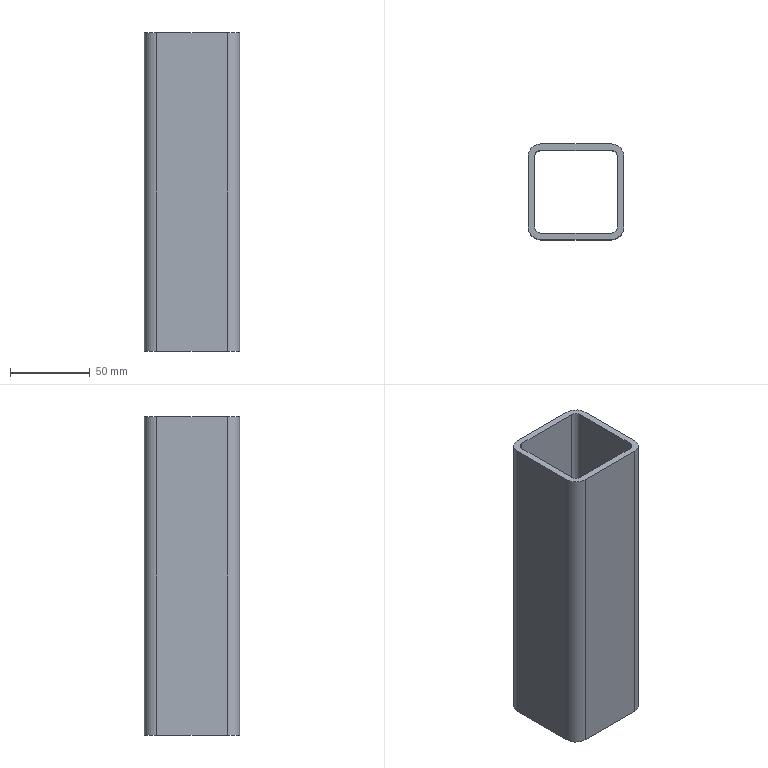Part | SolidWorks | features BaseBody 1 | 1 solid | 18 faces | box 60 x 60 x 200 mm | volume 170959 mm3 | plane 10 | cylinder 8 | commonest cylinder face diameters 8 x4 16 x4
STEP:
#1=CARTESIAN_POINT('',(696.,2440.,-1360.));
#2=VERTEX_POINT('',#1);
#3=CARTESIAN_POINT('',(696.,2484.,-1360.));
#4=VERTEX_POINT('',#3);
#5=CARTESIAN_POINT('',(696.,2440.,-1360.));
#6=DIRECTION('',(0.,1.,0.));
#7=VECTOR('',#6,1000.);
#8=LINE('',#5,#7);
#9=EDGE_CURVE('',#2,#4,#8,.T.);
#10=ORIENTED_EDGE('',*,*,#9,.T.);
#11=CARTESIAN_POINT('',(696.,2484.,-1560.));
#12=VERTEX_POINT('',#11);
#13=CARTESIAN_POINT('',(696.,2484.,-1530.));
#14=DIRECTION('',(0.,0.,-1.));
#15=VECTOR('',#14,1000.);
#16=LINE('',#13,#15);
#17=EDGE_CURVE('',#4,#12,#16,.T.);
#18=ORIENTED_EDGE('',*,*,#17,.T.);
#19=CARTESIAN_POINT('',(696.,2440.,-1560.));
#20=VERTEX_POINT('',#19);
#21=CARTESIAN_POINT('',(696.,2440.,-1560.));
#22=DIRECTION('',(0.,-1.,0.));
#23=VECTOR('',#22,1000.);
#24=LINE('',#21,#23);
#25=EDGE_CURVE('',#12,#20,#24,.T.);
#26=ORIENTED_EDGE('',*,*,#25,.T.);
#27=CARTESIAN_POINT('',(696.,2440.,-1530.));
#28=DIRECTION('',(0.,0.,1.));
#29=VECTOR('',#28,1000.);
#30=LINE('',#27,#29);
#31=EDGE_CURVE('',#20,#2,#30,.T.);
#32=ORIENTED_EDGE('',*,*,#31,.T.);
#33=EDGE_LOOP('',(#10,#18,#26,#32));
#34=FACE_OUTER_BOUND('',#33,.T.);
#35=CARTESIAN_POINT('',(696.,2440.,-1530.));
#36=DIRECTION('',(-1.,0.,0.));
#37=DIRECTION('',(0.,0.,1.));
#38=AXIS2_PLACEMENT_3D('',#35,#36,#37);
#39=PLANE('',#38);
#40=ADVANCED_FACE('',(#34),#39,.T.);
#41=ORIENTED_EDGE('',*,*,#17,.F.);
#42=CARTESIAN_POINT('',(692.,2488.,-1360.));
#43=VERTEX_POINT('',#42);
#44=CARTESIAN_POINT('',(692.,2484.,-1360.));
#45=DIRECTION('',(0.,0.,-1.));
#46=DIRECTION('',(1.,0.,0.));
#47=AXIS2_PLACEMENT_3D('',#44,#45,#46);
#48=CIRCLE('',#47,4.);
#49=EDGE_CURVE('',#43,#4,#48,.T.);
#50=ORIENTED_EDGE('',*,*,#49,.F.);
#51=CARTESIAN_POINT('',(692.,2488.,-1560.));
#52=VERTEX_POINT('',#51);
#53=CARTESIAN_POINT('',(692.,2488.,-1530.));
#54=DIRECTION('',(0.,0.,1.));
#55=VECTOR('',#54,1000.);
#56=LINE('',#53,#55);
#57=EDGE_CURVE('',#52,#43,#56,.T.);
#58=ORIENTED_EDGE('',*,*,#57,.F.);
#59=CARTESIAN_POINT('',(692.,2484.,-1560.));
#60=DIRECTION('',(0.,0.,1.));
#61=DIRECTION('',(1.,0.,0.));
#62=AXIS2_PLACEMENT_3D('',#59,#60,#61);
#63=CIRCLE('',#62,4.);
#64=EDGE_CURVE('',#12,#52,#63,.T.);
#65=ORIENTED_EDGE('',*,*,#64,.F.);
#66=EDGE_LOOP('',(#41,#50,#58,#65));
#67=FACE_OUTER_BOUND('',#66,.T.);
#68=CARTESIAN_POINT('',(692.,2484.,-1530.));
#69=DIRECTION('',(0.,0.,1.));
#70=DIRECTION('',(1.,0.,0.));
#71=AXIS2_PLACEMENT_3D('',#68,#69,#70);
#72=CYLINDRICAL_SURFACE('',#71,4.);
#73=ADVANCED_FACE('',(#67),#72,.F.);
#74=CARTESIAN_POINT('',(692.,2436.,-1360.));
#75=VERTEX_POINT('',#74);
#76=CARTESIAN_POINT('',(692.,2440.,-1360.));
#77=DIRECTION('',(0.,0.,1.));
#78=DIRECTION('',(1.,0.,0.));
#79=AXIS2_PLACEMENT_3D('',#76,#77,#78);
#80=CIRCLE('',#79,4.);
#81=EDGE_CURVE('',#75,#2,#80,.T.);
#82=ORIENTED_EDGE('',*,*,#81,.F.);
#83=CARTESIAN_POINT('',(648.,2436.,-1360.));
#84=VERTEX_POINT('',#83);
#85=CARTESIAN_POINT('',(-670.,2436.,-1360.));
#86=DIRECTION('',(1.,0.,0.));
#87=VECTOR('',#86,1000.);
#88=LINE('',#85,#87);
#89=EDGE_CURVE('',#84,#75,#88,.T.);
#90=ORIENTED_EDGE('',*,*,#89,.F.);
#91=CARTESIAN_POINT('',(644.,2440.,-1360.));
#92=VERTEX_POINT('',#91);
#93=CARTESIAN_POINT('',(648.,2440.,-1360.));
#94=DIRECTION('',(0.,0.,1.));
#95=DIRECTION('',(1.,0.,0.));
#96=AXIS2_PLACEMENT_3D('',#93,#94,#95);
#97=CIRCLE('',#96,4.);
#98=EDGE_CURVE('',#92,#84,#97,.T.);
#99=ORIENTED_EDGE('',*,*,#98,.F.);
#100=CARTESIAN_POINT('',(644.,2484.,-1360.));
#101=VERTEX_POINT('',#100);
#102=CARTESIAN_POINT('',(644.,1242.,-1360.));
#103=DIRECTION('',(0.,-1.,0.));
#104=VECTOR('',#103,1000.);
#105=LINE('',#102,#104);
#106=EDGE_CURVE('',#101,#92,#105,.T.);
#107=ORIENTED_EDGE('',*,*,#106,.F.);
#108=CARTESIAN_POINT('',(648.,2488.,-1360.));
#109=VERTEX_POINT('',#108);
#110=CARTESIAN_POINT('',(648.,2484.,-1360.));
#111=DIRECTION('',(0.,0.,1.));
#112=DIRECTION('',(1.,0.,0.));
#113=AXIS2_PLACEMENT_3D('',#110,#111,#112);
#114=CIRCLE('',#113,4.);
#115=EDGE_CURVE('',#109,#101,#114,.T.);
#116=ORIENTED_EDGE('',*,*,#115,.F.);
#117=CARTESIAN_POINT('',(-670.,2488.,-1360.));
#118=DIRECTION('',(-1.,0.,0.));
#119=VECTOR('',#118,1000.);
#120=LINE('',#117,#119);
#121=EDGE_CURVE('',#43,#109,#120,.T.);
#122=ORIENTED_EDGE('',*,*,#121,.F.);
#123=ORIENTED_EDGE('',*,*,#49,.T.);
#124=ORIENTED_EDGE('',*,*,#9,.F.);
#125=EDGE_LOOP('',(#82,#90,#99,#107,#116,#122,#123,#124));
#126=FACE_BOUND('',#125,.T.);
#127=CARTESIAN_POINT('',(692.,2432.,-1360.));
#128=VERTEX_POINT('',#127);
#129=CARTESIAN_POINT('',(648.,2432.,-1360.));
#130=VERTEX_POINT('',#129);
#131=CARTESIAN_POINT('',(-670.,2432.,-1360.));
#132=DIRECTION('',(-1.,0.,0.));
#133=VECTOR('',#132,1000.);
#134=LINE('',#131,#133);
#135=EDGE_CURVE('',#128,#130,#134,.T.);
#136=ORIENTED_EDGE('',*,*,#135,.F.);
#137=CARTESIAN_POINT('',(700.,2440.,-1360.));
#138=VERTEX_POINT('',#137);
#139=CARTESIAN_POINT('',(692.,2440.,-1360.));
#140=DIRECTION('',(0.,0.,-1.));
#141=DIRECTION('',(1.,0.,0.));
#142=AXIS2_PLACEMENT_3D('',#139,#140,#141);
#143=CIRCLE('',#142,8.);
#144=EDGE_CURVE('',#138,#128,#143,.T.);
#145=ORIENTED_EDGE('',*,*,#144,.F.);
#146=CARTESIAN_POINT('',(700.,2484.,-1360.));
#147=VERTEX_POINT('',#146);
#148=CARTESIAN_POINT('',(700.,1242.,-1360.));
#149=DIRECTION('',(0.,-1.,0.));
#150=VECTOR('',#149,1000.);
#151=LINE('',#148,#150);
#152=EDGE_CURVE('',#147,#138,#151,.T.);
#153=ORIENTED_EDGE('',*,*,#152,.F.);
#154=CARTESIAN_POINT('',(692.,2492.,-1360.));
#155=VERTEX_POINT('',#154);
#156=CARTESIAN_POINT('',(692.,2484.,-1360.));
#157=DIRECTION('',(0.,0.,-1.));
#158=DIRECTION('',(1.,0.,0.));
#159=AXIS2_PLACEMENT_3D('',#156,#157,#158);
#160=CIRCLE('',#159,8.);
#161=EDGE_CURVE('',#155,#147,#160,.T.);
#162=ORIENTED_EDGE('',*,*,#161,.F.);
#163=CARTESIAN_POINT('',(648.,2492.,-1360.));
#164=VERTEX_POINT('',#163);
#165=CARTESIAN_POINT('',(-670.,2492.,-1360.));
#166=DIRECTION('',(1.,0.,0.));
#167=VECTOR('',#166,1000.);
#168=LINE('',#165,#167);
#169=EDGE_CURVE('',#164,#155,#168,.T.);
#170=ORIENTED_EDGE('',*,*,#169,.F.);
#171=CARTESIAN_POINT('',(640.,2484.,-1360.));
#172=VERTEX_POINT('',#171);
#173=CARTESIAN_POINT('',(648.,2484.,-1360.));
#174=DIRECTION('',(0.,0.,-1.));
#175=DIRECTION('',(1.,0.,0.));
#176=AXIS2_PLACEMENT_3D('',#173,#174,#175);
#177=CIRCLE('',#176,8.);
#178=EDGE_CURVE('',#172,#164,#177,.T.);
#179=ORIENTED_EDGE('',*,*,#178,.F.);
#180=CARTESIAN_POINT('',(640.,2440.,-1360.));
#181=VERTEX_POINT('',#180);
#182=CARTESIAN_POINT('',(640.,1242.,-1360.));
#183=DIRECTION('',(0.,1.,0.));
#184=VECTOR('',#183,1000.);
#185=LINE('',#182,#184);
#186=EDGE_CURVE('',#181,#172,#185,.T.);
#187=ORIENTED_EDGE('',*,*,#186,.F.);
#188=CARTESIAN_POINT('',(648.,2440.,-1360.));
#189=DIRECTION('',(0.,0.,-1.));
#190=DIRECTION('',(1.,0.,0.));
#191=AXIS2_PLACEMENT_3D('',#188,#189,#190);
#192=CIRCLE('',#191,8.);
#193=EDGE_CURVE('',#130,#181,#192,.T.);
#194=ORIENTED_EDGE('',*,*,#193,.F.);
#195=EDGE_LOOP('',(#136,#145,#153,#162,#170,#179,#187,#194));
#196=FACE_OUTER_BOUND('',#195,.T.);
#197=CARTESIAN_POINT('',(-670.,1242.,-1360.));
#198=DIRECTION('',(0.,0.,-1.));
#199=DIRECTION('',(-1.,0.,0.));
#200=AXIS2_PLACEMENT_3D('',#197,#198,#199);
#201=PLANE('',#200);
#202=ADVANCED_FACE('',(#126,#196),#201,.F.);
#203=CARTESIAN_POINT('',(692.,2436.,-1560.));
#204=VERTEX_POINT('',#203);
#205=CARTESIAN_POINT('',(692.,2436.,-1530.));
#206=DIRECTION('',(0.,0.,-1.));
#207=VECTOR('',#206,1000.);
#208=LINE('',#205,#207);
#209=EDGE_CURVE('',#75,#204,#208,.T.);
#210=ORIENTED_EDGE('',*,*,#209,.F.);
#211=ORIENTED_EDGE('',*,*,#81,.T.);
#212=ORIENTED_EDGE('',*,*,#31,.F.);
#213=CARTESIAN_POINT('',(692.,2440.,-1560.));
#214=DIRECTION('',(0.,0.,1.));
#215=DIRECTION('',(1.,0.,0.));
#216=AXIS2_PLACEMENT_3D('',#213,#214,#215);
#217=CIRCLE('',#216,4.);
#218=EDGE_CURVE('',#204,#20,#217,.T.);
#219=ORIENTED_EDGE('',*,*,#218,.F.);
#220=EDGE_LOOP('',(#210,#211,#212,#219));
#221=FACE_OUTER_BOUND('',#220,.T.);
#222=CARTESIAN_POINT('',(692.,2440.,-1530.));
#223=DIRECTION('',(0.,0.,1.));
#224=DIRECTION('',(1.,0.,0.));
#225=AXIS2_PLACEMENT_3D('',#222,#223,#224);
#226=CYLINDRICAL_SURFACE('',#225,4.);
#227=ADVANCED_FACE('',(#221),#226,.F.);
#228=ORIENTED_EDGE('',*,*,#25,.F.);
#229=ORIENTED_EDGE('',*,*,#64,.T.);
#230=CARTESIAN_POINT('',(648.,2488.,-1560.));
#231=VERTEX_POINT('',#230);
#232=CARTESIAN_POINT('',(670.,2488.,-1560.));
#233=DIRECTION('',(-1.,0.,0.));
#234=VECTOR('',#233,1000.);
#235=LINE('',#232,#234);
#236=EDGE_CURVE('',#52,#231,#235,.T.);
#237=ORIENTED_EDGE('',*,*,#236,.T.);
#238=CARTESIAN_POINT('',(644.,2484.,-1560.));
#239=VERTEX_POINT('',#238);
#240=CARTESIAN_POINT('',(648.,2484.,-1560.));
#241=DIRECTION('',(0.,0.,1.));
#242=DIRECTION('',(1.,0.,0.));
#243=AXIS2_PLACEMENT_3D('',#240,#241,#242);
#244=CIRCLE('',#243,4.);
#245=EDGE_CURVE('',#231,#239,#244,.T.);
#246=ORIENTED_EDGE('',*,*,#245,.T.);
#247=CARTESIAN_POINT('',(644.,2440.,-1560.));
#248=VERTEX_POINT('',#247);
#249=CARTESIAN_POINT('',(644.,2492.,-1560.));
#250=DIRECTION('',(0.,-1.,0.));
#251=VECTOR('',#250,1000.);
#252=LINE('',#249,#251);
#253=EDGE_CURVE('',#239,#248,#252,.T.);
#254=ORIENTED_EDGE('',*,*,#253,.T.);
#255=CARTESIAN_POINT('',(648.,2436.,-1560.));
#256=VERTEX_POINT('',#255);
#257=CARTESIAN_POINT('',(648.,2440.,-1560.));
#258=DIRECTION('',(0.,0.,1.));
#259=DIRECTION('',(1.,0.,0.));
#260=AXIS2_PLACEMENT_3D('',#257,#258,#259);
#261=CIRCLE('',#260,4.);
#262=EDGE_CURVE('',#248,#256,#261,.T.);
#263=ORIENTED_EDGE('',*,*,#262,.T.);
#264=CARTESIAN_POINT('',(670.,2436.,-1560.));
#265=DIRECTION('',(1.,0.,0.));
#266=VECTOR('',#265,1000.);
#267=LINE('',#264,#266);
#268=EDGE_CURVE('',#256,#204,#267,.T.);
#269=ORIENTED_EDGE('',*,*,#268,.T.);
#270=ORIENTED_EDGE('',*,*,#218,.T.);
#271=EDGE_LOOP('',(#228,#229,#237,#246,#254,#263,#269,#270));
#272=FACE_BOUND('',#271,.T.);
#273=CARTESIAN_POINT('',(648.,2432.,-1560.));
#274=VERTEX_POINT('',#273);
#275=CARTESIAN_POINT('',(640.,2440.,-1560.));
#276=VERTEX_POINT('',#275);
#277=CARTESIAN_POINT('',(648.,2440.,-1560.));
#278=DIRECTION('',(0.,0.,-1.));
#279=DIRECTION('',(1.,0.,0.));
#280=AXIS2_PLACEMENT_3D('',#277,#278,#279);
#281=CIRCLE('',#280,8.);
#282=EDGE_CURVE('',#274,#276,#281,.T.);
#283=ORIENTED_EDGE('',*,*,#282,.T.);
#284=CARTESIAN_POINT('',(640.,2484.,-1560.));
#285=VERTEX_POINT('',#284);
#286=CARTESIAN_POINT('',(640.,2492.,-1560.));
#287=DIRECTION('',(0.,1.,0.));
#288=VECTOR('',#287,1000.);
#289=LINE('',#286,#288);
#290=EDGE_CURVE('',#276,#285,#289,.T.);
#291=ORIENTED_EDGE('',*,*,#290,.T.);
#292=CARTESIAN_POINT('',(648.,2492.,-1560.));
#293=VERTEX_POINT('',#292);
#294=CARTESIAN_POINT('',(648.,2484.,-1560.));
#295=DIRECTION('',(0.,0.,-1.));
#296=DIRECTION('',(1.,0.,0.));
#297=AXIS2_PLACEMENT_3D('',#294,#295,#296);
#298=CIRCLE('',#297,8.);
#299=EDGE_CURVE('',#285,#293,#298,.T.);
#300=ORIENTED_EDGE('',*,*,#299,.T.);
#301=CARTESIAN_POINT('',(692.,2492.,-1560.));
#302=VERTEX_POINT('',#301);
#303=CARTESIAN_POINT('',(670.,2492.,-1560.));
#304=DIRECTION('',(1.,0.,0.));
#305=VECTOR('',#304,1000.);
#306=LINE('',#303,#305);
#307=EDGE_CURVE('',#293,#302,#306,.T.);
#308=ORIENTED_EDGE('',*,*,#307,.T.);
#309=CARTESIAN_POINT('',(700.,2484.,-1560.));
#310=VERTEX_POINT('',#309);
#311=CARTESIAN_POINT('',(692.,2484.,-1560.));
#312=DIRECTION('',(0.,0.,-1.));
#313=DIRECTION('',(1.,0.,0.));
#314=AXIS2_PLACEMENT_3D('',#311,#312,#313);
#315=CIRCLE('',#314,8.);
#316=EDGE_CURVE('',#302,#310,#315,.T.);
#317=ORIENTED_EDGE('',*,*,#316,.T.);
#318=CARTESIAN_POINT('',(700.,2440.,-1560.));
#319=VERTEX_POINT('',#318);
#320=CARTESIAN_POINT('',(700.,2492.,-1560.));
#321=DIRECTION('',(0.,-1.,0.));
#322=VECTOR('',#321,1000.);
#323=LINE('',#320,#322);
#324=EDGE_CURVE('',#310,#319,#323,.T.);
#325=ORIENTED_EDGE('',*,*,#324,.T.);
#326=CARTESIAN_POINT('',(692.,2432.,-1560.));
#327=VERTEX_POINT('',#326);
#328=CARTESIAN_POINT('',(692.,2440.,-1560.));
#329=DIRECTION('',(0.,0.,-1.));
#330=DIRECTION('',(1.,0.,0.));
#331=AXIS2_PLACEMENT_3D('',#328,#329,#330);
#332=CIRCLE('',#331,8.);
#333=EDGE_CURVE('',#319,#327,#332,.T.);
#334=ORIENTED_EDGE('',*,*,#333,.T.);
#335=CARTESIAN_POINT('',(670.,2432.,-1560.));
#336=DIRECTION('',(-1.,0.,0.));
#337=VECTOR('',#336,1000.);
#338=LINE('',#335,#337);
#339=EDGE_CURVE('',#327,#274,#338,.T.);
#340=ORIENTED_EDGE('',*,*,#339,.T.);
#341=EDGE_LOOP('',(#283,#291,#300,#308,#317,#325,#334,#340));
#342=FACE_OUTER_BOUND('',#341,.T.);
#343=CARTESIAN_POINT('',(670.,2492.,-1560.));
#344=DIRECTION('',(0.,0.,-1.));
#345=DIRECTION('',(-1.,0.,0.));
#346=AXIS2_PLACEMENT_3D('',#343,#344,#345);
#347=PLANE('',#346);
#348=ADVANCED_FACE('',(#272,#342),#347,.T.);
#349=ORIENTED_EDGE('',*,*,#121,.T.);
#350=CARTESIAN_POINT('',(648.,2488.,-1530.));
#351=DIRECTION('',(0.,0.,-1.));
#352=VECTOR('',#351,1000.);
#353=LINE('',#350,#352);
#354=EDGE_CURVE('',#109,#231,#353,.T.);
#355=ORIENTED_EDGE('',*,*,#354,.T.);
#356=ORIENTED_EDGE('',*,*,#236,.F.);
#357=ORIENTED_EDGE('',*,*,#57,.T.);
#358=EDGE_LOOP('',(#349,#355,#356,#357));
#359=FACE_OUTER_BOUND('',#358,.T.);
#360=CARTESIAN_POINT('',(648.,2488.,-1530.));
#361=DIRECTION('',(0.,-1.,0.));
#362=DIRECTION('',(0.,0.,-1.));
#363=AXIS2_PLACEMENT_3D('',#360,#361,#362);
#364=PLANE('',#363);
#365=ADVANCED_FACE('',(#359),#364,.T.);
#366=ORIENTED_EDGE('',*,*,#89,.T.);
#367=ORIENTED_EDGE('',*,*,#209,.T.);
#368=ORIENTED_EDGE('',*,*,#268,.F.);
#369=CARTESIAN_POINT('',(648.,2436.,-1530.));
#370=DIRECTION('',(0.,0.,1.));
#371=VECTOR('',#370,1000.);
#372=LINE('',#369,#371);
#373=EDGE_CURVE('',#256,#84,#372,.T.);
#374=ORIENTED_EDGE('',*,*,#373,.T.);
#375=EDGE_LOOP('',(#366,#367,#368,#374));
#376=FACE_OUTER_BOUND('',#375,.T.);
#377=CARTESIAN_POINT('',(692.,2436.,-1530.));
#378=DIRECTION('',(0.,1.,0.));
#379=DIRECTION('',(0.,0.,1.));
#380=AXIS2_PLACEMENT_3D('',#377,#378,#379);
#381=PLANE('',#380);
#382=ADVANCED_FACE('',(#376),#381,.T.);
#383=CARTESIAN_POINT('',(644.,2440.,-1530.));
#384=DIRECTION('',(0.,0.,-1.));
#385=VECTOR('',#384,1000.);
#386=LINE('',#383,#385);
#387=EDGE_CURVE('',#92,#248,#386,.T.);
#388=ORIENTED_EDGE('',*,*,#387,.F.);
#389=ORIENTED_EDGE('',*,*,#98,.T.);
#390=ORIENTED_EDGE('',*,*,#373,.F.);
#391=ORIENTED_EDGE('',*,*,#262,.F.);
#392=EDGE_LOOP('',(#388,#389,#390,#391));
#393=FACE_OUTER_BOUND('',#392,.T.);
#394=CARTESIAN_POINT('',(648.,2440.,-1530.));
#395=DIRECTION('',(0.,0.,1.));
#396=DIRECTION('',(1.,0.,0.));
#397=AXIS2_PLACEMENT_3D('',#394,#395,#396);
#398=CYLINDRICAL_SURFACE('',#397,4.);
#399=ADVANCED_FACE('',(#393),#398,.F.);
#400=ORIENTED_EDGE('',*,*,#106,.T.);
#401=ORIENTED_EDGE('',*,*,#387,.T.);
#402=ORIENTED_EDGE('',*,*,#253,.F.);
#403=CARTESIAN_POINT('',(644.,2484.,-1530.));
#404=DIRECTION('',(0.,0.,1.));
#405=VECTOR('',#404,1000.);
#406=LINE('',#403,#405);
#407=EDGE_CURVE('',#239,#101,#406,.T.);
#408=ORIENTED_EDGE('',*,*,#407,.T.);
#409=EDGE_LOOP('',(#400,#401,#402,#408));
#410=FACE_OUTER_BOUND('',#409,.T.);
#411=CARTESIAN_POINT('',(644.,2484.,-1530.));
#412=DIRECTION('',(1.,0.,0.));
#413=DIRECTION('',(0.,0.,-1.));
#414=AXIS2_PLACEMENT_3D('',#411,#412,#413);
#415=PLANE('',#414);
#416=ADVANCED_FACE('',(#410),#415,.T.);
#417=ORIENTED_EDGE('',*,*,#354,.F.);
#418=ORIENTED_EDGE('',*,*,#115,.T.);
#419=ORIENTED_EDGE('',*,*,#407,.F.);
#420=ORIENTED_EDGE('',*,*,#245,.F.);
#421=EDGE_LOOP('',(#417,#418,#419,#420));
#422=FACE_OUTER_BOUND('',#421,.T.);
#423=CARTESIAN_POINT('',(648.,2484.,-1530.));
#424=DIRECTION('',(0.,0.,1.));
#425=DIRECTION('',(1.,0.,0.));
#426=AXIS2_PLACEMENT_3D('',#423,#424,#425);
#427=CYLINDRICAL_SURFACE('',#426,4.);
#428=ADVANCED_FACE('',(#422),#427,.F.);
#429=CARTESIAN_POINT('',(640.,2440.,-1530.));
#430=DIRECTION('',(0.,0.,-1.));
#431=VECTOR('',#430,1000.);
#432=LINE('',#429,#431);
#433=EDGE_CURVE('',#181,#276,#432,.T.);
#434=ORIENTED_EDGE('',*,*,#433,.T.);
#435=ORIENTED_EDGE('',*,*,#282,.F.);
#436=CARTESIAN_POINT('',(648.,2432.,-1530.));
#437=DIRECTION('',(0.,0.,1.));
#438=VECTOR('',#437,1000.);
#439=LINE('',#436,#438);
#440=EDGE_CURVE('',#274,#130,#439,.T.);
#441=ORIENTED_EDGE('',*,*,#440,.T.);
#442=ORIENTED_EDGE('',*,*,#193,.T.);
#443=EDGE_LOOP('',(#434,#435,#441,#442));
#444=FACE_OUTER_BOUND('',#443,.T.);
#445=CARTESIAN_POINT('',(648.,2440.,-1530.));
#446=DIRECTION('',(0.,0.,1.));
#447=DIRECTION('',(1.,0.,0.));
#448=AXIS2_PLACEMENT_3D('',#445,#446,#447);
#449=CYLINDRICAL_SURFACE('',#448,8.);
#450=ADVANCED_FACE('',(#444),#449,.T.);
#451=ORIENTED_EDGE('',*,*,#135,.T.);
#452=ORIENTED_EDGE('',*,*,#440,.F.);
#453=ORIENTED_EDGE('',*,*,#339,.F.);
#454=CARTESIAN_POINT('',(692.,2432.,-1530.));
#455=DIRECTION('',(0.,0.,-1.));
#456=VECTOR('',#455,1000.);
#457=LINE('',#454,#456);
#458=EDGE_CURVE('',#128,#327,#457,.T.);
#459=ORIENTED_EDGE('',*,*,#458,.F.);
#460=EDGE_LOOP('',(#451,#452,#453,#459));
#461=FACE_OUTER_BOUND('',#460,.T.);
#462=CARTESIAN_POINT('',(692.,2432.,-1530.));
#463=DIRECTION('',(0.,1.,0.));
#464=DIRECTION('',(0.,0.,1.));
#465=AXIS2_PLACEMENT_3D('',#462,#463,#464);
#466=PLANE('',#465);
#467=ADVANCED_FACE('',(#461),#466,.F.);
#468=ORIENTED_EDGE('',*,*,#458,.T.);
#469=ORIENTED_EDGE('',*,*,#333,.F.);
#470=CARTESIAN_POINT('',(700.,2440.,-1530.));
#471=DIRECTION('',(0.,0.,1.));
#472=VECTOR('',#471,1000.);
#473=LINE('',#470,#472);
#474=EDGE_CURVE('',#319,#138,#473,.T.);
#475=ORIENTED_EDGE('',*,*,#474,.T.);
#476=ORIENTED_EDGE('',*,*,#144,.T.);
#477=EDGE_LOOP('',(#468,#469,#475,#476));
#478=FACE_OUTER_BOUND('',#477,.T.);
#479=CARTESIAN_POINT('',(692.,2440.,-1530.));
#480=DIRECTION('',(0.,0.,1.));
#481=DIRECTION('',(1.,0.,0.));
#482=AXIS2_PLACEMENT_3D('',#479,#480,#481);
#483=CYLINDRICAL_SURFACE('',#482,8.);
#484=ADVANCED_FACE('',(#478),#483,.T.);
#485=ORIENTED_EDGE('',*,*,#152,.T.);
#486=ORIENTED_EDGE('',*,*,#474,.F.);
#487=ORIENTED_EDGE('',*,*,#324,.F.);
#488=CARTESIAN_POINT('',(700.,2484.,-1530.));
#489=DIRECTION('',(0.,0.,-1.));
#490=VECTOR('',#489,1000.);
#491=LINE('',#488,#490);
#492=EDGE_CURVE('',#147,#310,#491,.T.);
#493=ORIENTED_EDGE('',*,*,#492,.F.);
#494=EDGE_LOOP('',(#485,#486,#487,#493));
#495=FACE_OUTER_BOUND('',#494,.T.);
#496=CARTESIAN_POINT('',(700.,2440.,-1530.));
#497=DIRECTION('',(-1.,0.,0.));
#498=DIRECTION('',(0.,0.,1.));
#499=AXIS2_PLACEMENT_3D('',#496,#497,#498);
#500=PLANE('',#499);
#501=ADVANCED_FACE('',(#495),#500,.F.);
#502=ORIENTED_EDGE('',*,*,#492,.T.);
#503=ORIENTED_EDGE('',*,*,#316,.F.);
#504=CARTESIAN_POINT('',(692.,2492.,-1530.));
#505=DIRECTION('',(0.,0.,1.));
#506=VECTOR('',#505,1000.);
#507=LINE('',#504,#506);
#508=EDGE_CURVE('',#302,#155,#507,.T.);
#509=ORIENTED_EDGE('',*,*,#508,.T.);
#510=ORIENTED_EDGE('',*,*,#161,.T.);
#511=EDGE_LOOP('',(#502,#503,#509,#510));
#512=FACE_OUTER_BOUND('',#511,.T.);
#513=CARTESIAN_POINT('',(692.,2484.,-1530.));
#514=DIRECTION('',(0.,0.,1.));
#515=DIRECTION('',(1.,0.,0.));
#516=AXIS2_PLACEMENT_3D('',#513,#514,#515);
#517=CYLINDRICAL_SURFACE('',#516,8.);
#518=ADVANCED_FACE('',(#512),#517,.T.);
#519=ORIENTED_EDGE('',*,*,#169,.T.);
#520=ORIENTED_EDGE('',*,*,#508,.F.);
#521=ORIENTED_EDGE('',*,*,#307,.F.);
#522=CARTESIAN_POINT('',(648.,2492.,-1530.));
#523=DIRECTION('',(0.,0.,-1.));
#524=VECTOR('',#523,1000.);
#525=LINE('',#522,#524);
#526=EDGE_CURVE('',#164,#293,#525,.T.);
#527=ORIENTED_EDGE('',*,*,#526,.F.);
#528=EDGE_LOOP('',(#519,#520,#521,#527));
#529=FACE_OUTER_BOUND('',#528,.T.);
#530=CARTESIAN_POINT('',(648.,2492.,-1530.));
#531=DIRECTION('',(0.,-1.,0.));
#532=DIRECTION('',(0.,0.,-1.));
#533=AXIS2_PLACEMENT_3D('',#530,#531,#532);
#534=PLANE('',#533);
#535=ADVANCED_FACE('',(#529),#534,.F.);
#536=ORIENTED_EDGE('',*,*,#526,.T.);
#537=ORIENTED_EDGE('',*,*,#299,.F.);
#538=CARTESIAN_POINT('',(640.,2484.,-1530.));
#539=DIRECTION('',(0.,0.,1.));
#540=VECTOR('',#539,1000.);
#541=LINE('',#538,#540);
#542=EDGE_CURVE('',#285,#172,#541,.T.);
#543=ORIENTED_EDGE('',*,*,#542,.T.);
#544=ORIENTED_EDGE('',*,*,#178,.T.);
#545=EDGE_LOOP('',(#536,#537,#543,#544));
#546=FACE_OUTER_BOUND('',#545,.T.);
#547=CARTESIAN_POINT('',(648.,2484.,-1530.));
#548=DIRECTION('',(0.,0.,1.));
#549=DIRECTION('',(1.,0.,0.));
#550=AXIS2_PLACEMENT_3D('',#547,#548,#549);
#551=CYLINDRICAL_SURFACE('',#550,8.);
#552=ADVANCED_FACE('',(#546),#551,.T.);
#553=ORIENTED_EDGE('',*,*,#186,.T.);
#554=ORIENTED_EDGE('',*,*,#542,.F.);
#555=ORIENTED_EDGE('',*,*,#290,.F.);
#556=ORIENTED_EDGE('',*,*,#433,.F.);
#557=EDGE_LOOP('',(#553,#554,#555,#556));
#558=FACE_OUTER_BOUND('',#557,.T.);
#559=CARTESIAN_POINT('',(640.,2484.,-1530.));
#560=DIRECTION('',(1.,0.,0.));
#561=DIRECTION('',(0.,0.,-1.));
#562=AXIS2_PLACEMENT_3D('',#559,#560,#561);
#563=PLANE('',#562);
#564=ADVANCED_FACE('',(#558),#563,.F.);
#565=CLOSED_SHELL('',(#40,#73,#202,#227,#348,#365,#382,#399,#416,#428,#450,#467,#484,#501,#518,#535,#552,#564));
#566=MANIFOLD_SOLID_BREP('',#565);
#567=CARTESIAN_POINT('',(0.,0.,0.));
#568=DIRECTION('',(0.,0.,1.));
#569=DIRECTION('',(1.,0.,0.));
#570=AXIS2_PLACEMENT_3D('',#567,#568,#569);
#571=(LENGTH_UNIT()NAMED_UNIT(*)SI_UNIT(.MILLI.,.METRE.));
#572=UNCERTAINTY_MEASURE_WITH_UNIT(LENGTH_MEASURE(0.00001),#571,'','');
#573=(NAMED_UNIT(*)PLANE_ANGLE_UNIT()SI_UNIT($,.RADIAN.));
#574=(NAMED_UNIT(*)SI_UNIT($,.STERADIAN.)SOLID_ANGLE_UNIT());
#575=(GEOMETRIC_REPRESENTATION_CONTEXT(3)GLOBAL_UNCERTAINTY_ASSIGNED_CONTEXT((#572))GLOBAL_UNIT_ASSIGNED_CONTEXT((#571,#573,#574))REPRESENTATION_CONTEXT('',''));
#576=ADVANCED_BREP_SHAPE_REPRESENTATION('',(#566,#570),#575);